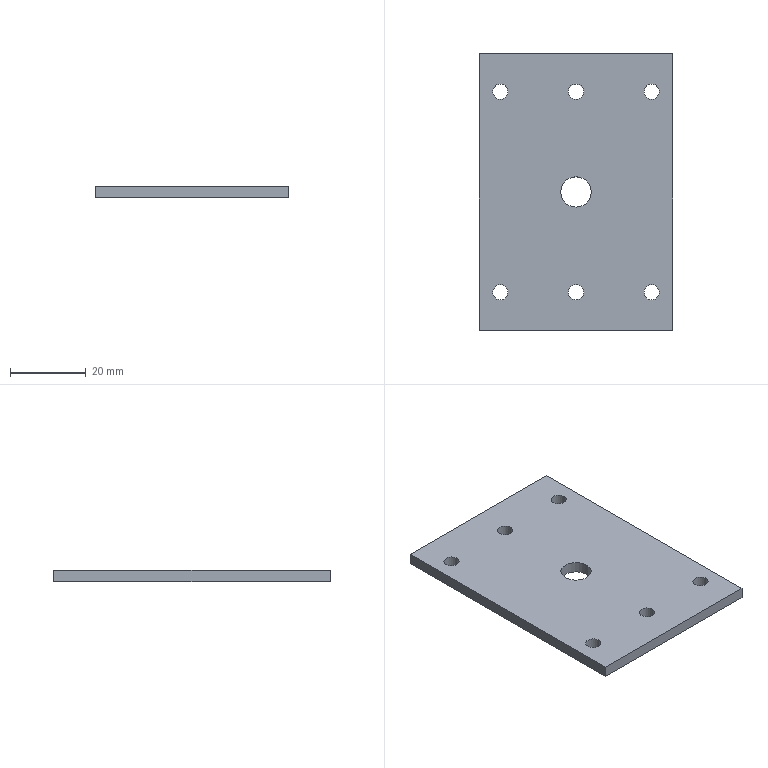Part | STEP file | 1-01.7 | 1 solid | 13 faces | box 51 x 73 x 3 mm | volume 10792 mm3 | cylinder 7 | plane 6 | commonest cylinder face diameters 4 x6 8 x1
STEP:
#1=CARTESIAN_POINT('',(0.,0.,0.));
#2=DIRECTION('',(0.,0.,1.));
#3=DIRECTION('',(1.,0.,0.));
#4=AXIS2_PLACEMENT_3D('',#1,#2,#3);
#5=CARTESIAN_POINT('',(25.5,-36.5,0.));
#6=VERTEX_POINT('',#5);
#7=CARTESIAN_POINT('',(25.5,36.5,0.));
#8=VERTEX_POINT('',#7);
#9=CARTESIAN_POINT('',(25.5,-36.5,0.));
#10=DIRECTION('',(0.,1.,0.));
#11=VECTOR('',#10,1.);
#12=LINE('',#9,#11);
#13=CARTESIAN_POINT('',(-11.,0.,0.));
#14=DIRECTION('',(0.,0.,1.));
#15=DIRECTION('',(0.,1.,0.));
#16=AXIS2_PLACEMENT_3D('',#13,#14,#15);
#17=PLANE('',#16);
#18=CARTESIAN_POINT('',(-36.5,-36.5));
#19=DIRECTION('',(1.,0.));
#20=VECTOR('',#19,1.);
#21=LINE('',#18,#20);
#22=(GEOMETRIC_REPRESENTATION_CONTEXT(2)PARAMETRIC_REPRESENTATION_CONTEXT()REPRESENTATION_CONTEXT('',''));
#23=DEFINITIONAL_REPRESENTATION('',(#21),#22);
#24=PCURVE('',#17,#23);
#25=CARTESIAN_POINT('',(25.5,0.,-1.5));
#26=DIRECTION('',(-1.,0.,0.));
#27=DIRECTION('',(0.,1.,0.));
#28=AXIS2_PLACEMENT_3D('',#25,#26,#27);
#29=PLANE('',#28);
#30=CARTESIAN_POINT('',(-36.5,-1.5));
#31=DIRECTION('',(1.,0.));
#32=VECTOR('',#31,1.);
#33=LINE('',#30,#32);
#34=(GEOMETRIC_REPRESENTATION_CONTEXT(2)PARAMETRIC_REPRESENTATION_CONTEXT()REPRESENTATION_CONTEXT('',''));
#35=DEFINITIONAL_REPRESENTATION('',(#33),#34);
#36=PCURVE('',#29,#35);
#37=SURFACE_CURVE('',#12,(#24,#36),.PCURVE_S1.);
#38=EDGE_CURVE('',#6,#8,#37,.T.);
#39=ORIENTED_EDGE('',*,*,#38,.T.);
#40=CARTESIAN_POINT('',(-25.5,36.5,0.));
#41=VERTEX_POINT('',#40);
#42=CARTESIAN_POINT('',(25.5,36.5,0.));
#43=DIRECTION('',(-1.,0.,0.));
#44=VECTOR('',#43,1.);
#45=LINE('',#42,#44);
#46=CARTESIAN_POINT('',(36.5,-36.5));
#47=DIRECTION('',(0.,1.));
#48=VECTOR('',#47,1.);
#49=LINE('',#46,#48);
#50=(GEOMETRIC_REPRESENTATION_CONTEXT(2)PARAMETRIC_REPRESENTATION_CONTEXT()REPRESENTATION_CONTEXT('',''));
#51=DEFINITIONAL_REPRESENTATION('',(#49),#50);
#52=PCURVE('',#17,#51);
#53=CARTESIAN_POINT('',(0.,36.5,-1.5));
#54=DIRECTION('',(0.,-1.,0.));
#55=DIRECTION('',(-1.,0.,0.));
#56=AXIS2_PLACEMENT_3D('',#53,#54,#55);
#57=PLANE('',#56);
#58=CARTESIAN_POINT('',(-25.5,-1.5));
#59=DIRECTION('',(1.,0.));
#60=VECTOR('',#59,1.);
#61=LINE('',#58,#60);
#62=(GEOMETRIC_REPRESENTATION_CONTEXT(2)PARAMETRIC_REPRESENTATION_CONTEXT()REPRESENTATION_CONTEXT('',''));
#63=DEFINITIONAL_REPRESENTATION('',(#61),#62);
#64=PCURVE('',#57,#63);
#65=SURFACE_CURVE('',#45,(#52,#64),.PCURVE_S1.);
#66=EDGE_CURVE('',#8,#41,#65,.T.);
#67=ORIENTED_EDGE('',*,*,#66,.T.);
#68=CARTESIAN_POINT('',(-25.5,-36.5,0.));
#69=VERTEX_POINT('',#68);
#70=CARTESIAN_POINT('',(-25.5,36.5,0.));
#71=DIRECTION('',(0.,-1.,0.));
#72=VECTOR('',#71,1.);
#73=LINE('',#70,#72);
#74=CARTESIAN_POINT('',(36.5,14.5));
#75=DIRECTION('',(-1.,0.));
#76=VECTOR('',#75,1.);
#77=LINE('',#74,#76);
#78=(GEOMETRIC_REPRESENTATION_CONTEXT(2)PARAMETRIC_REPRESENTATION_CONTEXT()REPRESENTATION_CONTEXT('',''));
#79=DEFINITIONAL_REPRESENTATION('',(#77),#78);
#80=PCURVE('',#17,#79);
#81=CARTESIAN_POINT('',(-25.5,0.,-1.5));
#82=DIRECTION('',(1.,0.,0.));
#83=DIRECTION('',(0.,-1.,0.));
#84=AXIS2_PLACEMENT_3D('',#81,#82,#83);
#85=PLANE('',#84);
#86=CARTESIAN_POINT('',(-36.5,-1.5));
#87=DIRECTION('',(1.,0.));
#88=VECTOR('',#87,1.);
#89=LINE('',#86,#88);
#90=(GEOMETRIC_REPRESENTATION_CONTEXT(2)PARAMETRIC_REPRESENTATION_CONTEXT()REPRESENTATION_CONTEXT('',''));
#91=DEFINITIONAL_REPRESENTATION('',(#89),#90);
#92=PCURVE('',#85,#91);
#93=SURFACE_CURVE('',#73,(#80,#92),.PCURVE_S1.);
#94=EDGE_CURVE('',#41,#69,#93,.T.);
#95=ORIENTED_EDGE('',*,*,#94,.T.);
#96=CARTESIAN_POINT('',(-25.5,-36.5,0.));
#97=DIRECTION('',(1.,0.,0.));
#98=VECTOR('',#97,1.);
#99=LINE('',#96,#98);
#100=CARTESIAN_POINT('',(-36.5,14.5));
#101=DIRECTION('',(0.,-1.));
#102=VECTOR('',#101,1.);
#103=LINE('',#100,#102);
#104=(GEOMETRIC_REPRESENTATION_CONTEXT(2)PARAMETRIC_REPRESENTATION_CONTEXT()REPRESENTATION_CONTEXT('',''));
#105=DEFINITIONAL_REPRESENTATION('',(#103),#104);
#106=PCURVE('',#17,#105);
#107=CARTESIAN_POINT('',(0.,-36.5,-1.5));
#108=DIRECTION('',(0.,1.,0.));
#109=DIRECTION('',(1.,0.,0.));
#110=AXIS2_PLACEMENT_3D('',#107,#108,#109);
#111=PLANE('',#110);
#112=CARTESIAN_POINT('',(-25.5,-1.5));
#113=DIRECTION('',(1.,0.));
#114=VECTOR('',#113,1.);
#115=LINE('',#112,#114);
#116=(GEOMETRIC_REPRESENTATION_CONTEXT(2)PARAMETRIC_REPRESENTATION_CONTEXT()REPRESENTATION_CONTEXT('',''));
#117=DEFINITIONAL_REPRESENTATION('',(#115),#116);
#118=PCURVE('',#111,#117);
#119=SURFACE_CURVE('',#99,(#106,#118),.PCURVE_S1.);
#120=EDGE_CURVE('',#69,#6,#119,.T.);
#121=ORIENTED_EDGE('',*,*,#120,.T.);
#122=EDGE_LOOP('',(#39,#67,#95,#121));
#123=FACE_BOUND('',#122,.T.);
#124=CARTESIAN_POINT('',(-20.,-24.5,0.));
#125=VERTEX_POINT('',#124);
#126=CARTESIAN_POINT('',(-20.,-26.5,0.));
#127=DIRECTION('',(0.,0.,-1.));
#128=DIRECTION('',(0.,1.,0.));
#129=AXIS2_PLACEMENT_3D('',#126,#127,#128);
#130=CIRCLE('',#129,2.);
#131=CARTESIAN_POINT('',(-24.5,9.));
#132=CARTESIAN_POINT('',(-24.5,5.536));
#133=CARTESIAN_POINT('',(-27.5,7.268));
#134=CARTESIAN_POINT('',(-30.5,9.));
#135=CARTESIAN_POINT('',(-27.5,10.732));
#136=CARTESIAN_POINT('',(-24.5,12.464));
#137=CARTESIAN_POINT('',(-24.5,9.));
#138=(BOUNDED_CURVE()B_SPLINE_CURVE(2,(#131,#132,#133,#134,#135,#136,#137),.UNSPECIFIED.,.T.,.F.)B_SPLINE_CURVE_WITH_KNOTS((1,2,2,2,2,1),(-2.094,0.,2.094,4.189,6.283,8.378),.UNSPECIFIED.)CURVE()GEOMETRIC_REPRESENTATION_ITEM()RATIONAL_B_SPLINE_CURVE((1.,0.5,1.,0.5,1.,0.5,1.))REPRESENTATION_ITEM(''));
#139=(GEOMETRIC_REPRESENTATION_CONTEXT(2)PARAMETRIC_REPRESENTATION_CONTEXT()REPRESENTATION_CONTEXT('',''));
#140=DEFINITIONAL_REPRESENTATION('',(#138),#139);
#141=PCURVE('',#17,#140);
#142=CARTESIAN_POINT('',(-20.,-26.5,0.));
#143=DIRECTION('',(0.,0.,-1.));
#144=DIRECTION('',(0.,1.,0.));
#145=AXIS2_PLACEMENT_3D('',#142,#143,#144);
#146=CYLINDRICAL_SURFACE('',#145,2.);
#147=CARTESIAN_POINT('',(0.,0.));
#148=DIRECTION('',(1.,0.));
#149=VECTOR('',#148,1.);
#150=LINE('',#147,#149);
#151=(GEOMETRIC_REPRESENTATION_CONTEXT(2)PARAMETRIC_REPRESENTATION_CONTEXT()REPRESENTATION_CONTEXT('',''));
#152=DEFINITIONAL_REPRESENTATION('',(#150),#151);
#153=PCURVE('',#146,#152);
#154=SURFACE_CURVE('',#130,(#141,#153),.PCURVE_S1.);
#155=EDGE_CURVE('',#125,#125,#154,.T.);
#156=ORIENTED_EDGE('',*,*,#155,.T.);
#157=EDGE_LOOP('',(#156));
#158=FACE_BOUND('',#157,.T.);
#159=CARTESIAN_POINT('',(0.,-24.5,0.));
#160=VERTEX_POINT('',#159);
#161=CARTESIAN_POINT('',(0.,-26.5,0.));
#162=DIRECTION('',(0.,0.,-1.));
#163=DIRECTION('',(0.,1.,0.));
#164=AXIS2_PLACEMENT_3D('',#161,#162,#163);
#165=CIRCLE('',#164,2.);
#166=CARTESIAN_POINT('',(-24.5,-11.));
#167=CARTESIAN_POINT('',(-24.5,-14.464));
#168=CARTESIAN_POINT('',(-27.5,-12.732));
#169=CARTESIAN_POINT('',(-30.5,-11.));
#170=CARTESIAN_POINT('',(-27.5,-9.268));
#171=CARTESIAN_POINT('',(-24.5,-7.536));
#172=CARTESIAN_POINT('',(-24.5,-11.));
#173=(BOUNDED_CURVE()B_SPLINE_CURVE(2,(#166,#167,#168,#169,#170,#171,#172),.UNSPECIFIED.,.T.,.F.)B_SPLINE_CURVE_WITH_KNOTS((1,2,2,2,2,1),(-2.094,0.,2.094,4.189,6.283,8.378),.UNSPECIFIED.)CURVE()GEOMETRIC_REPRESENTATION_ITEM()RATIONAL_B_SPLINE_CURVE((1.,0.5,1.,0.5,1.,0.5,1.))REPRESENTATION_ITEM(''));
#174=(GEOMETRIC_REPRESENTATION_CONTEXT(2)PARAMETRIC_REPRESENTATION_CONTEXT()REPRESENTATION_CONTEXT('',''));
#175=DEFINITIONAL_REPRESENTATION('',(#173),#174);
#176=PCURVE('',#17,#175);
#177=CARTESIAN_POINT('',(0.,-26.5,0.));
#178=DIRECTION('',(0.,0.,-1.));
#179=DIRECTION('',(0.,1.,0.));
#180=AXIS2_PLACEMENT_3D('',#177,#178,#179);
#181=CYLINDRICAL_SURFACE('',#180,2.);
#182=CARTESIAN_POINT('',(0.,0.));
#183=DIRECTION('',(1.,0.));
#184=VECTOR('',#183,1.);
#185=LINE('',#182,#184);
#186=(GEOMETRIC_REPRESENTATION_CONTEXT(2)PARAMETRIC_REPRESENTATION_CONTEXT()REPRESENTATION_CONTEXT('',''));
#187=DEFINITIONAL_REPRESENTATION('',(#185),#186);
#188=PCURVE('',#181,#187);
#189=SURFACE_CURVE('',#165,(#176,#188),.PCURVE_S1.);
#190=EDGE_CURVE('',#160,#160,#189,.T.);
#191=ORIENTED_EDGE('',*,*,#190,.T.);
#192=EDGE_LOOP('',(#191));
#193=FACE_BOUND('',#192,.T.);
#194=CARTESIAN_POINT('',(0.,4.,0.));
#195=VERTEX_POINT('',#194);
#196=CARTESIAN_POINT('',(0.,0.,0.));
#197=DIRECTION('',(0.,0.,-1.));
#198=DIRECTION('',(0.,1.,0.));
#199=AXIS2_PLACEMENT_3D('',#196,#197,#198);
#200=CIRCLE('',#199,4.);
#201=CARTESIAN_POINT('',(4.,-11.));
#202=CARTESIAN_POINT('',(4.,-17.928));
#203=CARTESIAN_POINT('',(-2.,-14.464));
#204=CARTESIAN_POINT('',(-8.,-11.));
#205=CARTESIAN_POINT('',(-2.,-7.536));
#206=CARTESIAN_POINT('',(4.,-4.072));
#207=CARTESIAN_POINT('',(4.,-11.));
#208=(BOUNDED_CURVE()B_SPLINE_CURVE(2,(#201,#202,#203,#204,#205,#206,#207),.UNSPECIFIED.,.T.,.F.)B_SPLINE_CURVE_WITH_KNOTS((1,2,2,2,2,1),(-2.094,0.,2.094,4.189,6.283,8.378),.UNSPECIFIED.)CURVE()GEOMETRIC_REPRESENTATION_ITEM()RATIONAL_B_SPLINE_CURVE((1.,0.5,1.,0.5,1.,0.5,1.))REPRESENTATION_ITEM(''));
#209=(GEOMETRIC_REPRESENTATION_CONTEXT(2)PARAMETRIC_REPRESENTATION_CONTEXT()REPRESENTATION_CONTEXT('',''));
#210=DEFINITIONAL_REPRESENTATION('',(#208),#209);
#211=PCURVE('',#17,#210);
#212=CARTESIAN_POINT('',(0.,0.,0.));
#213=DIRECTION('',(0.,0.,-1.));
#214=DIRECTION('',(0.,1.,0.));
#215=AXIS2_PLACEMENT_3D('',#212,#213,#214);
#216=CYLINDRICAL_SURFACE('',#215,4.);
#217=CARTESIAN_POINT('',(0.,0.));
#218=DIRECTION('',(1.,0.));
#219=VECTOR('',#218,1.);
#220=LINE('',#217,#219);
#221=(GEOMETRIC_REPRESENTATION_CONTEXT(2)PARAMETRIC_REPRESENTATION_CONTEXT()REPRESENTATION_CONTEXT('',''));
#222=DEFINITIONAL_REPRESENTATION('',(#220),#221);
#223=PCURVE('',#216,#222);
#224=SURFACE_CURVE('',#200,(#211,#223),.PCURVE_S1.);
#225=EDGE_CURVE('',#195,#195,#224,.T.);
#226=ORIENTED_EDGE('',*,*,#225,.T.);
#227=EDGE_LOOP('',(#226));
#228=FACE_BOUND('',#227,.T.);
#229=CARTESIAN_POINT('',(20.,-24.5,0.));
#230=VERTEX_POINT('',#229);
#231=CARTESIAN_POINT('',(20.,-26.5,0.));
#232=DIRECTION('',(0.,0.,-1.));
#233=DIRECTION('',(0.,1.,0.));
#234=AXIS2_PLACEMENT_3D('',#231,#232,#233);
#235=CIRCLE('',#234,2.);
#236=CARTESIAN_POINT('',(-24.5,-31.));
#237=CARTESIAN_POINT('',(-24.5,-34.464));
#238=CARTESIAN_POINT('',(-27.5,-32.732));
#239=CARTESIAN_POINT('',(-30.5,-31.));
#240=CARTESIAN_POINT('',(-27.5,-29.268));
#241=CARTESIAN_POINT('',(-24.5,-27.536));
#242=CARTESIAN_POINT('',(-24.5,-31.));
#243=(BOUNDED_CURVE()B_SPLINE_CURVE(2,(#236,#237,#238,#239,#240,#241,#242),.UNSPECIFIED.,.T.,.F.)B_SPLINE_CURVE_WITH_KNOTS((1,2,2,2,2,1),(-2.094,0.,2.094,4.189,6.283,8.378),.UNSPECIFIED.)CURVE()GEOMETRIC_REPRESENTATION_ITEM()RATIONAL_B_SPLINE_CURVE((1.,0.5,1.,0.5,1.,0.5,1.))REPRESENTATION_ITEM(''));
#244=(GEOMETRIC_REPRESENTATION_CONTEXT(2)PARAMETRIC_REPRESENTATION_CONTEXT()REPRESENTATION_CONTEXT('',''));
#245=DEFINITIONAL_REPRESENTATION('',(#243),#244);
#246=PCURVE('',#17,#245);
#247=CARTESIAN_POINT('',(20.,-26.5,0.));
#248=DIRECTION('',(0.,0.,-1.));
#249=DIRECTION('',(0.,1.,0.));
#250=AXIS2_PLACEMENT_3D('',#247,#248,#249);
#251=CYLINDRICAL_SURFACE('',#250,2.);
#252=CARTESIAN_POINT('',(0.,0.));
#253=DIRECTION('',(1.,0.));
#254=VECTOR('',#253,1.);
#255=LINE('',#252,#254);
#256=(GEOMETRIC_REPRESENTATION_CONTEXT(2)PARAMETRIC_REPRESENTATION_CONTEXT()REPRESENTATION_CONTEXT('',''));
#257=DEFINITIONAL_REPRESENTATION('',(#255),#256);
#258=PCURVE('',#251,#257);
#259=SURFACE_CURVE('',#235,(#246,#258),.PCURVE_S1.);
#260=EDGE_CURVE('',#230,#230,#259,.T.);
#261=ORIENTED_EDGE('',*,*,#260,.T.);
#262=EDGE_LOOP('',(#261));
#263=FACE_BOUND('',#262,.T.);
#264=CARTESIAN_POINT('',(-20.,28.5,0.));
#265=VERTEX_POINT('',#264);
#266=CARTESIAN_POINT('',(-20.,26.5,0.));
#267=DIRECTION('',(0.,0.,-1.));
#268=DIRECTION('',(0.,1.,0.));
#269=AXIS2_PLACEMENT_3D('',#266,#267,#268);
#270=CIRCLE('',#269,2.);
#271=CARTESIAN_POINT('',(28.5,9.));
#272=CARTESIAN_POINT('',(28.5,5.536));
#273=CARTESIAN_POINT('',(25.5,7.268));
#274=CARTESIAN_POINT('',(22.5,9.));
#275=CARTESIAN_POINT('',(25.5,10.732));
#276=CARTESIAN_POINT('',(28.5,12.464));
#277=CARTESIAN_POINT('',(28.5,9.));
#278=(BOUNDED_CURVE()B_SPLINE_CURVE(2,(#271,#272,#273,#274,#275,#276,#277),.UNSPECIFIED.,.T.,.F.)B_SPLINE_CURVE_WITH_KNOTS((1,2,2,2,2,1),(-2.094,0.,2.094,4.189,6.283,8.378),.UNSPECIFIED.)CURVE()GEOMETRIC_REPRESENTATION_ITEM()RATIONAL_B_SPLINE_CURVE((1.,0.5,1.,0.5,1.,0.5,1.))REPRESENTATION_ITEM(''));
#279=(GEOMETRIC_REPRESENTATION_CONTEXT(2)PARAMETRIC_REPRESENTATION_CONTEXT()REPRESENTATION_CONTEXT('',''));
#280=DEFINITIONAL_REPRESENTATION('',(#278),#279);
#281=PCURVE('',#17,#280);
#282=CARTESIAN_POINT('',(-20.,26.5,0.));
#283=DIRECTION('',(0.,0.,-1.));
#284=DIRECTION('',(0.,1.,0.));
#285=AXIS2_PLACEMENT_3D('',#282,#283,#284);
#286=CYLINDRICAL_SURFACE('',#285,2.);
#287=CARTESIAN_POINT('',(0.,0.));
#288=DIRECTION('',(1.,0.));
#289=VECTOR('',#288,1.);
#290=LINE('',#287,#289);
#291=(GEOMETRIC_REPRESENTATION_CONTEXT(2)PARAMETRIC_REPRESENTATION_CONTEXT()REPRESENTATION_CONTEXT('',''));
#292=DEFINITIONAL_REPRESENTATION('',(#290),#291);
#293=PCURVE('',#286,#292);
#294=SURFACE_CURVE('',#270,(#281,#293),.PCURVE_S1.);
#295=EDGE_CURVE('',#265,#265,#294,.T.);
#296=ORIENTED_EDGE('',*,*,#295,.T.);
#297=EDGE_LOOP('',(#296));
#298=FACE_BOUND('',#297,.T.);
#299=CARTESIAN_POINT('',(0.,28.5,0.));
#300=VERTEX_POINT('',#299);
#301=CARTESIAN_POINT('',(0.,26.5,0.));
#302=DIRECTION('',(0.,0.,-1.));
#303=DIRECTION('',(0.,1.,0.));
#304=AXIS2_PLACEMENT_3D('',#301,#302,#303);
#305=CIRCLE('',#304,2.);
#306=CARTESIAN_POINT('',(28.5,-11.));
#307=CARTESIAN_POINT('',(28.5,-14.464));
#308=CARTESIAN_POINT('',(25.5,-12.732));
#309=CARTESIAN_POINT('',(22.5,-11.));
#310=CARTESIAN_POINT('',(25.5,-9.268));
#311=CARTESIAN_POINT('',(28.5,-7.536));
#312=CARTESIAN_POINT('',(28.5,-11.));
#313=(BOUNDED_CURVE()B_SPLINE_CURVE(2,(#306,#307,#308,#309,#310,#311,#312),.UNSPECIFIED.,.T.,.F.)B_SPLINE_CURVE_WITH_KNOTS((1,2,2,2,2,1),(-2.094,0.,2.094,4.189,6.283,8.378),.UNSPECIFIED.)CURVE()GEOMETRIC_REPRESENTATION_ITEM()RATIONAL_B_SPLINE_CURVE((1.,0.5,1.,0.5,1.,0.5,1.))REPRESENTATION_ITEM(''));
#314=(GEOMETRIC_REPRESENTATION_CONTEXT(2)PARAMETRIC_REPRESENTATION_CONTEXT()REPRESENTATION_CONTEXT('',''));
#315=DEFINITIONAL_REPRESENTATION('',(#313),#314);
#316=PCURVE('',#17,#315);
#317=CARTESIAN_POINT('',(0.,26.5,0.));
#318=DIRECTION('',(0.,0.,-1.));
#319=DIRECTION('',(0.,1.,0.));
#320=AXIS2_PLACEMENT_3D('',#317,#318,#319);
#321=CYLINDRICAL_SURFACE('',#320,2.);
#322=CARTESIAN_POINT('',(0.,0.));
#323=DIRECTION('',(1.,0.));
#324=VECTOR('',#323,1.);
#325=LINE('',#322,#324);
#326=(GEOMETRIC_REPRESENTATION_CONTEXT(2)PARAMETRIC_REPRESENTATION_CONTEXT()REPRESENTATION_CONTEXT('',''));
#327=DEFINITIONAL_REPRESENTATION('',(#325),#326);
#328=PCURVE('',#321,#327);
#329=SURFACE_CURVE('',#305,(#316,#328),.PCURVE_S1.);
#330=EDGE_CURVE('',#300,#300,#329,.T.);
#331=ORIENTED_EDGE('',*,*,#330,.T.);
#332=EDGE_LOOP('',(#331));
#333=FACE_BOUND('',#332,.T.);
#334=CARTESIAN_POINT('',(20.,28.5,0.));
#335=VERTEX_POINT('',#334);
#336=CARTESIAN_POINT('',(20.,26.5,0.));
#337=DIRECTION('',(0.,0.,-1.));
#338=DIRECTION('',(0.,1.,0.));
#339=AXIS2_PLACEMENT_3D('',#336,#337,#338);
#340=CIRCLE('',#339,2.);
#341=CARTESIAN_POINT('',(28.5,-31.));
#342=CARTESIAN_POINT('',(28.5,-34.464));
#343=CARTESIAN_POINT('',(25.5,-32.732));
#344=CARTESIAN_POINT('',(22.5,-31.));
#345=CARTESIAN_POINT('',(25.5,-29.268));
#346=CARTESIAN_POINT('',(28.5,-27.536));
#347=CARTESIAN_POINT('',(28.5,-31.));
#348=(BOUNDED_CURVE()B_SPLINE_CURVE(2,(#341,#342,#343,#344,#345,#346,#347),.UNSPECIFIED.,.T.,.F.)B_SPLINE_CURVE_WITH_KNOTS((1,2,2,2,2,1),(-2.094,0.,2.094,4.189,6.283,8.378),.UNSPECIFIED.)CURVE()GEOMETRIC_REPRESENTATION_ITEM()RATIONAL_B_SPLINE_CURVE((1.,0.5,1.,0.5,1.,0.5,1.))REPRESENTATION_ITEM(''));
#349=(GEOMETRIC_REPRESENTATION_CONTEXT(2)PARAMETRIC_REPRESENTATION_CONTEXT()REPRESENTATION_CONTEXT('',''));
#350=DEFINITIONAL_REPRESENTATION('',(#348),#349);
#351=PCURVE('',#17,#350);
#352=CARTESIAN_POINT('',(20.,26.5,0.));
#353=DIRECTION('',(0.,0.,-1.));
#354=DIRECTION('',(0.,1.,0.));
#355=AXIS2_PLACEMENT_3D('',#352,#353,#354);
#356=CYLINDRICAL_SURFACE('',#355,2.);
#357=CARTESIAN_POINT('',(0.,0.));
#358=DIRECTION('',(1.,0.));
#359=VECTOR('',#358,1.);
#360=LINE('',#357,#359);
#361=(GEOMETRIC_REPRESENTATION_CONTEXT(2)PARAMETRIC_REPRESENTATION_CONTEXT()REPRESENTATION_CONTEXT('',''));
#362=DEFINITIONAL_REPRESENTATION('',(#360),#361);
#363=PCURVE('',#356,#362);
#364=SURFACE_CURVE('',#340,(#351,#363),.PCURVE_S1.);
#365=EDGE_CURVE('',#335,#335,#364,.T.);
#366=ORIENTED_EDGE('',*,*,#365,.T.);
#367=EDGE_LOOP('',(#366));
#368=FACE_BOUND('',#367,.T.);
#369=ADVANCED_FACE('',(#123,#158,#193,#228,#263,#298,#333,#368),#17,.T.);
#370=CARTESIAN_POINT('',(25.5,-36.5,-3.));
#371=VERTEX_POINT('',#370);
#372=CARTESIAN_POINT('',(25.5,36.5,-3.));
#373=VERTEX_POINT('',#372);
#374=CARTESIAN_POINT('',(25.5,-36.5,-3.));
#375=DIRECTION('',(0.,1.,0.));
#376=VECTOR('',#375,1.);
#377=LINE('',#374,#376);
#378=CARTESIAN_POINT('',(-11.,0.,-3.));
#379=DIRECTION('',(0.,0.,1.));
#380=DIRECTION('',(0.,1.,0.));
#381=AXIS2_PLACEMENT_3D('',#378,#379,#380);
#382=PLANE('',#381);
#383=CARTESIAN_POINT('',(-36.5,-36.5));
#384=DIRECTION('',(1.,0.));
#385=VECTOR('',#384,1.);
#386=LINE('',#383,#385);
#387=(GEOMETRIC_REPRESENTATION_CONTEXT(2)PARAMETRIC_REPRESENTATION_CONTEXT()REPRESENTATION_CONTEXT('',''));
#388=DEFINITIONAL_REPRESENTATION('',(#386),#387);
#389=PCURVE('',#382,#388);
#390=CARTESIAN_POINT('',(-36.5,1.5));
#391=DIRECTION('',(1.,0.));
#392=VECTOR('',#391,1.);
#393=LINE('',#390,#392);
#394=(GEOMETRIC_REPRESENTATION_CONTEXT(2)PARAMETRIC_REPRESENTATION_CONTEXT()REPRESENTATION_CONTEXT('',''));
#395=DEFINITIONAL_REPRESENTATION('',(#393),#394);
#396=PCURVE('',#29,#395);
#397=SURFACE_CURVE('',#377,(#389,#396),.PCURVE_S1.);
#398=EDGE_CURVE('',#371,#373,#397,.T.);
#399=ORIENTED_EDGE('',*,*,#398,.T.);
#400=CARTESIAN_POINT('',(-25.5,36.5,-3.));
#401=VERTEX_POINT('',#400);
#402=CARTESIAN_POINT('',(25.5,36.5,-3.));
#403=DIRECTION('',(-1.,0.,0.));
#404=VECTOR('',#403,1.);
#405=LINE('',#402,#404);
#406=CARTESIAN_POINT('',(36.5,-36.5));
#407=DIRECTION('',(0.,1.));
#408=VECTOR('',#407,1.);
#409=LINE('',#406,#408);
#410=(GEOMETRIC_REPRESENTATION_CONTEXT(2)PARAMETRIC_REPRESENTATION_CONTEXT()REPRESENTATION_CONTEXT('',''));
#411=DEFINITIONAL_REPRESENTATION('',(#409),#410);
#412=PCURVE('',#382,#411);
#413=CARTESIAN_POINT('',(-25.5,1.5));
#414=DIRECTION('',(1.,0.));
#415=VECTOR('',#414,1.);
#416=LINE('',#413,#415);
#417=(GEOMETRIC_REPRESENTATION_CONTEXT(2)PARAMETRIC_REPRESENTATION_CONTEXT()REPRESENTATION_CONTEXT('',''));
#418=DEFINITIONAL_REPRESENTATION('',(#416),#417);
#419=PCURVE('',#57,#418);
#420=SURFACE_CURVE('',#405,(#412,#419),.PCURVE_S1.);
#421=EDGE_CURVE('',#373,#401,#420,.T.);
#422=ORIENTED_EDGE('',*,*,#421,.T.);
#423=CARTESIAN_POINT('',(-25.5,-36.5,-3.));
#424=VERTEX_POINT('',#423);
#425=CARTESIAN_POINT('',(-25.5,36.5,-3.));
#426=DIRECTION('',(0.,-1.,0.));
#427=VECTOR('',#426,1.);
#428=LINE('',#425,#427);
#429=CARTESIAN_POINT('',(36.5,14.5));
#430=DIRECTION('',(-1.,0.));
#431=VECTOR('',#430,1.);
#432=LINE('',#429,#431);
#433=(GEOMETRIC_REPRESENTATION_CONTEXT(2)PARAMETRIC_REPRESENTATION_CONTEXT()REPRESENTATION_CONTEXT('',''));
#434=DEFINITIONAL_REPRESENTATION('',(#432),#433);
#435=PCURVE('',#382,#434);
#436=CARTESIAN_POINT('',(-36.5,1.5));
#437=DIRECTION('',(1.,0.));
#438=VECTOR('',#437,1.);
#439=LINE('',#436,#438);
#440=(GEOMETRIC_REPRESENTATION_CONTEXT(2)PARAMETRIC_REPRESENTATION_CONTEXT()REPRESENTATION_CONTEXT('',''));
#441=DEFINITIONAL_REPRESENTATION('',(#439),#440);
#442=PCURVE('',#85,#441);
#443=SURFACE_CURVE('',#428,(#435,#442),.PCURVE_S1.);
#444=EDGE_CURVE('',#401,#424,#443,.T.);
#445=ORIENTED_EDGE('',*,*,#444,.T.);
#446=CARTESIAN_POINT('',(-25.5,-36.5,-3.));
#447=DIRECTION('',(1.,0.,0.));
#448=VECTOR('',#447,1.);
#449=LINE('',#446,#448);
#450=CARTESIAN_POINT('',(-36.5,14.5));
#451=DIRECTION('',(0.,-1.));
#452=VECTOR('',#451,1.);
#453=LINE('',#450,#452);
#454=(GEOMETRIC_REPRESENTATION_CONTEXT(2)PARAMETRIC_REPRESENTATION_CONTEXT()REPRESENTATION_CONTEXT('',''));
#455=DEFINITIONAL_REPRESENTATION('',(#453),#454);
#456=PCURVE('',#382,#455);
#457=CARTESIAN_POINT('',(-25.5,1.5));
#458=DIRECTION('',(1.,0.));
#459=VECTOR('',#458,1.);
#460=LINE('',#457,#459);
#461=(GEOMETRIC_REPRESENTATION_CONTEXT(2)PARAMETRIC_REPRESENTATION_CONTEXT()REPRESENTATION_CONTEXT('',''));
#462=DEFINITIONAL_REPRESENTATION('',(#460),#461);
#463=PCURVE('',#111,#462);
#464=SURFACE_CURVE('',#449,(#456,#463),.PCURVE_S1.);
#465=EDGE_CURVE('',#424,#371,#464,.T.);
#466=ORIENTED_EDGE('',*,*,#465,.T.);
#467=EDGE_LOOP('',(#399,#422,#445,#466));
#468=FACE_BOUND('',#467,.F.);
#469=CARTESIAN_POINT('',(-20.,-24.5,-3.));
#470=VERTEX_POINT('',#469);
#471=CARTESIAN_POINT('',(-20.,-26.5,-3.));
#472=DIRECTION('',(0.,0.,-1.));
#473=DIRECTION('',(0.,1.,0.));
#474=AXIS2_PLACEMENT_3D('',#471,#472,#473);
#475=CIRCLE('',#474,2.);
#476=CARTESIAN_POINT('',(-24.5,9.));
#477=CARTESIAN_POINT('',(-24.5,5.536));
#478=CARTESIAN_POINT('',(-27.5,7.268));
#479=CARTESIAN_POINT('',(-30.5,9.));
#480=CARTESIAN_POINT('',(-27.5,10.732));
#481=CARTESIAN_POINT('',(-24.5,12.464));
#482=CARTESIAN_POINT('',(-24.5,9.));
#483=(BOUNDED_CURVE()B_SPLINE_CURVE(2,(#476,#477,#478,#479,#480,#481,#482),.UNSPECIFIED.,.T.,.F.)B_SPLINE_CURVE_WITH_KNOTS((1,2,2,2,2,1),(-2.094,0.,2.094,4.189,6.283,8.378),.UNSPECIFIED.)CURVE()GEOMETRIC_REPRESENTATION_ITEM()RATIONAL_B_SPLINE_CURVE((1.,0.5,1.,0.5,1.,0.5,1.))REPRESENTATION_ITEM(''));
#484=(GEOMETRIC_REPRESENTATION_CONTEXT(2)PARAMETRIC_REPRESENTATION_CONTEXT()REPRESENTATION_CONTEXT('',''));
#485=DEFINITIONAL_REPRESENTATION('',(#483),#484);
#486=PCURVE('',#382,#485);
#487=CARTESIAN_POINT('',(0.,3.));
#488=DIRECTION('',(1.,0.));
#489=VECTOR('',#488,1.);
#490=LINE('',#487,#489);
#491=(GEOMETRIC_REPRESENTATION_CONTEXT(2)PARAMETRIC_REPRESENTATION_CONTEXT()REPRESENTATION_CONTEXT('',''));
#492=DEFINITIONAL_REPRESENTATION('',(#490),#491);
#493=PCURVE('',#146,#492);
#494=SURFACE_CURVE('',#475,(#486,#493),.PCURVE_S1.);
#495=EDGE_CURVE('',#470,#470,#494,.T.);
#496=ORIENTED_EDGE('',*,*,#495,.T.);
#497=EDGE_LOOP('',(#496));
#498=FACE_BOUND('',#497,.F.);
#499=CARTESIAN_POINT('',(0.,-24.5,-3.));
#500=VERTEX_POINT('',#499);
#501=CARTESIAN_POINT('',(0.,-26.5,-3.));
#502=DIRECTION('',(0.,0.,-1.));
#503=DIRECTION('',(0.,1.,0.));
#504=AXIS2_PLACEMENT_3D('',#501,#502,#503);
#505=CIRCLE('',#504,2.);
#506=CARTESIAN_POINT('',(-24.5,-11.));
#507=CARTESIAN_POINT('',(-24.5,-14.464));
#508=CARTESIAN_POINT('',(-27.5,-12.732));
#509=CARTESIAN_POINT('',(-30.5,-11.));
#510=CARTESIAN_POINT('',(-27.5,-9.268));
#511=CARTESIAN_POINT('',(-24.5,-7.536));
#512=CARTESIAN_POINT('',(-24.5,-11.));
#513=(BOUNDED_CURVE()B_SPLINE_CURVE(2,(#506,#507,#508,#509,#510,#511,#512),.UNSPECIFIED.,.T.,.F.)B_SPLINE_CURVE_WITH_KNOTS((1,2,2,2,2,1),(-2.094,0.,2.094,4.189,6.283,8.378),.UNSPECIFIED.)CURVE()GEOMETRIC_REPRESENTATION_ITEM()RATIONAL_B_SPLINE_CURVE((1.,0.5,1.,0.5,1.,0.5,1.))REPRESENTATION_ITEM(''));
#514=(GEOMETRIC_REPRESENTATION_CONTEXT(2)PARAMETRIC_REPRESENTATION_CONTEXT()REPRESENTATION_CONTEXT('',''));
#515=DEFINITIONAL_REPRESENTATION('',(#513),#514);
#516=PCURVE('',#382,#515);
#517=CARTESIAN_POINT('',(0.,3.));
#518=DIRECTION('',(1.,0.));
#519=VECTOR('',#518,1.);
#520=LINE('',#517,#519);
#521=(GEOMETRIC_REPRESENTATION_CONTEXT(2)PARAMETRIC_REPRESENTATION_CONTEXT()REPRESENTATION_CONTEXT('',''));
#522=DEFINITIONAL_REPRESENTATION('',(#520),#521);
#523=PCURVE('',#181,#522);
#524=SURFACE_CURVE('',#505,(#516,#523),.PCURVE_S1.);
#525=EDGE_CURVE('',#500,#500,#524,.T.);
#526=ORIENTED_EDGE('',*,*,#525,.T.);
#527=EDGE_LOOP('',(#526));
#528=FACE_BOUND('',#527,.F.);
#529=CARTESIAN_POINT('',(0.,4.,-3.));
#530=VERTEX_POINT('',#529);
#531=CARTESIAN_POINT('',(0.,0.,-3.));
#532=DIRECTION('',(0.,0.,-1.));
#533=DIRECTION('',(0.,1.,0.));
#534=AXIS2_PLACEMENT_3D('',#531,#532,#533);
#535=CIRCLE('',#534,4.);
#536=CARTESIAN_POINT('',(4.,-11.));
#537=CARTESIAN_POINT('',(4.,-17.928));
#538=CARTESIAN_POINT('',(-2.,-14.464));
#539=CARTESIAN_POINT('',(-8.,-11.));
#540=CARTESIAN_POINT('',(-2.,-7.536));
#541=CARTESIAN_POINT('',(4.,-4.072));
#542=CARTESIAN_POINT('',(4.,-11.));
#543=(BOUNDED_CURVE()B_SPLINE_CURVE(2,(#536,#537,#538,#539,#540,#541,#542),.UNSPECIFIED.,.T.,.F.)B_SPLINE_CURVE_WITH_KNOTS((1,2,2,2,2,1),(-2.094,0.,2.094,4.189,6.283,8.378),.UNSPECIFIED.)CURVE()GEOMETRIC_REPRESENTATION_ITEM()RATIONAL_B_SPLINE_CURVE((1.,0.5,1.,0.5,1.,0.5,1.))REPRESENTATION_ITEM(''));
#544=(GEOMETRIC_REPRESENTATION_CONTEXT(2)PARAMETRIC_REPRESENTATION_CONTEXT()REPRESENTATION_CONTEXT('',''));
#545=DEFINITIONAL_REPRESENTATION('',(#543),#544);
#546=PCURVE('',#382,#545);
#547=CARTESIAN_POINT('',(0.,3.));
#548=DIRECTION('',(1.,0.));
#549=VECTOR('',#548,1.);
#550=LINE('',#547,#549);
#551=(GEOMETRIC_REPRESENTATION_CONTEXT(2)PARAMETRIC_REPRESENTATION_CONTEXT()REPRESENTATION_CONTEXT('',''));
#552=DEFINITIONAL_REPRESENTATION('',(#550),#551);
#553=PCURVE('',#216,#552);
#554=SURFACE_CURVE('',#535,(#546,#553),.PCURVE_S1.);
#555=EDGE_CURVE('',#530,#530,#554,.T.);
#556=ORIENTED_EDGE('',*,*,#555,.T.);
#557=EDGE_LOOP('',(#556));
#558=FACE_BOUND('',#557,.F.);
#559=CARTESIAN_POINT('',(20.,-24.5,-3.));
#560=VERTEX_POINT('',#559);
#561=CARTESIAN_POINT('',(20.,-26.5,-3.));
#562=DIRECTION('',(0.,0.,-1.));
#563=DIRECTION('',(0.,1.,0.));
#564=AXIS2_PLACEMENT_3D('',#561,#562,#563);
#565=CIRCLE('',#564,2.);
#566=CARTESIAN_POINT('',(-24.5,-31.));
#567=CARTESIAN_POINT('',(-24.5,-34.464));
#568=CARTESIAN_POINT('',(-27.5,-32.732));
#569=CARTESIAN_POINT('',(-30.5,-31.));
#570=CARTESIAN_POINT('',(-27.5,-29.268));
#571=CARTESIAN_POINT('',(-24.5,-27.536));
#572=CARTESIAN_POINT('',(-24.5,-31.));
#573=(BOUNDED_CURVE()B_SPLINE_CURVE(2,(#566,#567,#568,#569,#570,#571,#572),.UNSPECIFIED.,.T.,.F.)B_SPLINE_CURVE_WITH_KNOTS((1,2,2,2,2,1),(-2.094,0.,2.094,4.189,6.283,8.378),.UNSPECIFIED.)CURVE()GEOMETRIC_REPRESENTATION_ITEM()RATIONAL_B_SPLINE_CURVE((1.,0.5,1.,0.5,1.,0.5,1.))REPRESENTATION_ITEM(''));
#574=(GEOMETRIC_REPRESENTATION_CONTEXT(2)PARAMETRIC_REPRESENTATION_CONTEXT()REPRESENTATION_CONTEXT('',''));
#575=DEFINITIONAL_REPRESENTATION('',(#573),#574);
#576=PCURVE('',#382,#575);
#577=CARTESIAN_POINT('',(0.,3.));
#578=DIRECTION('',(1.,0.));
#579=VECTOR('',#578,1.);
#580=LINE('',#577,#579);
#581=(GEOMETRIC_REPRESENTATION_CONTEXT(2)PARAMETRIC_REPRESENTATION_CONTEXT()REPRESENTATION_CONTEXT('',''));
#582=DEFINITIONAL_REPRESENTATION('',(#580),#581);
#583=PCURVE('',#251,#582);
#584=SURFACE_CURVE('',#565,(#576,#583),.PCURVE_S1.);
#585=EDGE_CURVE('',#560,#560,#584,.T.);
#586=ORIENTED_EDGE('',*,*,#585,.T.);
#587=EDGE_LOOP('',(#586));
#588=FACE_BOUND('',#587,.F.);
#589=CARTESIAN_POINT('',(-20.,28.5,-3.));
#590=VERTEX_POINT('',#589);
#591=CARTESIAN_POINT('',(-20.,26.5,-3.));
#592=DIRECTION('',(0.,0.,-1.));
#593=DIRECTION('',(0.,1.,0.));
#594=AXIS2_PLACEMENT_3D('',#591,#592,#593);
#595=CIRCLE('',#594,2.);
#596=CARTESIAN_POINT('',(28.5,9.));
#597=CARTESIAN_POINT('',(28.5,5.536));
#598=CARTESIAN_POINT('',(25.5,7.268));
#599=CARTESIAN_POINT('',(22.5,9.));
#600=CARTESIAN_POINT('',(25.5,10.732));
#601=CARTESIAN_POINT('',(28.5,12.464));
#602=CARTESIAN_POINT('',(28.5,9.));
#603=(BOUNDED_CURVE()B_SPLINE_CURVE(2,(#596,#597,#598,#599,#600,#601,#602),.UNSPECIFIED.,.T.,.F.)B_SPLINE_CURVE_WITH_KNOTS((1,2,2,2,2,1),(-2.094,0.,2.094,4.189,6.283,8.378),.UNSPECIFIED.)CURVE()GEOMETRIC_REPRESENTATION_ITEM()RATIONAL_B_SPLINE_CURVE((1.,0.5,1.,0.5,1.,0.5,1.))REPRESENTATION_ITEM(''));
#604=(GEOMETRIC_REPRESENTATION_CONTEXT(2)PARAMETRIC_REPRESENTATION_CONTEXT()REPRESENTATION_CONTEXT('',''));
#605=DEFINITIONAL_REPRESENTATION('',(#603),#604);
#606=PCURVE('',#382,#605);
#607=CARTESIAN_POINT('',(0.,3.));
#608=DIRECTION('',(1.,0.));
#609=VECTOR('',#608,1.);
#610=LINE('',#607,#609);
#611=(GEOMETRIC_REPRESENTATION_CONTEXT(2)PARAMETRIC_REPRESENTATION_CONTEXT()REPRESENTATION_CONTEXT('',''));
#612=DEFINITIONAL_REPRESENTATION('',(#610),#611);
#613=PCURVE('',#286,#612);
#614=SURFACE_CURVE('',#595,(#606,#613),.PCURVE_S1.);
#615=EDGE_CURVE('',#590,#590,#614,.T.);
#616=ORIENTED_EDGE('',*,*,#615,.T.);
#617=EDGE_LOOP('',(#616));
#618=FACE_BOUND('',#617,.F.);
#619=CARTESIAN_POINT('',(0.,28.5,-3.));
#620=VERTEX_POINT('',#619);
#621=CARTESIAN_POINT('',(0.,26.5,-3.));
#622=DIRECTION('',(0.,0.,-1.));
#623=DIRECTION('',(0.,1.,0.));
#624=AXIS2_PLACEMENT_3D('',#621,#622,#623);
#625=CIRCLE('',#624,2.);
#626=CARTESIAN_POINT('',(28.5,-11.));
#627=CARTESIAN_POINT('',(28.5,-14.464));
#628=CARTESIAN_POINT('',(25.5,-12.732));
#629=CARTESIAN_POINT('',(22.5,-11.));
#630=CARTESIAN_POINT('',(25.5,-9.268));
#631=CARTESIAN_POINT('',(28.5,-7.536));
#632=CARTESIAN_POINT('',(28.5,-11.));
#633=(BOUNDED_CURVE()B_SPLINE_CURVE(2,(#626,#627,#628,#629,#630,#631,#632),.UNSPECIFIED.,.T.,.F.)B_SPLINE_CURVE_WITH_KNOTS((1,2,2,2,2,1),(-2.094,0.,2.094,4.189,6.283,8.378),.UNSPECIFIED.)CURVE()GEOMETRIC_REPRESENTATION_ITEM()RATIONAL_B_SPLINE_CURVE((1.,0.5,1.,0.5,1.,0.5,1.))REPRESENTATION_ITEM(''));
#634=(GEOMETRIC_REPRESENTATION_CONTEXT(2)PARAMETRIC_REPRESENTATION_CONTEXT()REPRESENTATION_CONTEXT('',''));
#635=DEFINITIONAL_REPRESENTATION('',(#633),#634);
#636=PCURVE('',#382,#635);
#637=CARTESIAN_POINT('',(0.,3.));
#638=DIRECTION('',(1.,0.));
#639=VECTOR('',#638,1.);
#640=LINE('',#637,#639);
#641=(GEOMETRIC_REPRESENTATION_CONTEXT(2)PARAMETRIC_REPRESENTATION_CONTEXT()REPRESENTATION_CONTEXT('',''));
#642=DEFINITIONAL_REPRESENTATION('',(#640),#641);
#643=PCURVE('',#321,#642);
#644=SURFACE_CURVE('',#625,(#636,#643),.PCURVE_S1.);
#645=EDGE_CURVE('',#620,#620,#644,.T.);
#646=ORIENTED_EDGE('',*,*,#645,.T.);
#647=EDGE_LOOP('',(#646));
#648=FACE_BOUND('',#647,.F.);
#649=CARTESIAN_POINT('',(20.,28.5,-3.));
#650=VERTEX_POINT('',#649);
#651=CARTESIAN_POINT('',(20.,26.5,-3.));
#652=DIRECTION('',(0.,0.,-1.));
#653=DIRECTION('',(0.,1.,0.));
#654=AXIS2_PLACEMENT_3D('',#651,#652,#653);
#655=CIRCLE('',#654,2.);
#656=CARTESIAN_POINT('',(28.5,-31.));
#657=CARTESIAN_POINT('',(28.5,-34.464));
#658=CARTESIAN_POINT('',(25.5,-32.732));
#659=CARTESIAN_POINT('',(22.5,-31.));
#660=CARTESIAN_POINT('',(25.5,-29.268));
#661=CARTESIAN_POINT('',(28.5,-27.536));
#662=CARTESIAN_POINT('',(28.5,-31.));
#663=(BOUNDED_CURVE()B_SPLINE_CURVE(2,(#656,#657,#658,#659,#660,#661,#662),.UNSPECIFIED.,.T.,.F.)B_SPLINE_CURVE_WITH_KNOTS((1,2,2,2,2,1),(-2.094,0.,2.094,4.189,6.283,8.378),.UNSPECIFIED.)CURVE()GEOMETRIC_REPRESENTATION_ITEM()RATIONAL_B_SPLINE_CURVE((1.,0.5,1.,0.5,1.,0.5,1.))REPRESENTATION_ITEM(''));
#664=(GEOMETRIC_REPRESENTATION_CONTEXT(2)PARAMETRIC_REPRESENTATION_CONTEXT()REPRESENTATION_CONTEXT('',''));
#665=DEFINITIONAL_REPRESENTATION('',(#663),#664);
#666=PCURVE('',#382,#665);
#667=CARTESIAN_POINT('',(0.,3.));
#668=DIRECTION('',(1.,0.));
#669=VECTOR('',#668,1.);
#670=LINE('',#667,#669);
#671=(GEOMETRIC_REPRESENTATION_CONTEXT(2)PARAMETRIC_REPRESENTATION_CONTEXT()REPRESENTATION_CONTEXT('',''));
#672=DEFINITIONAL_REPRESENTATION('',(#670),#671);
#673=PCURVE('',#356,#672);
#674=SURFACE_CURVE('',#655,(#666,#673),.PCURVE_S1.);
#675=EDGE_CURVE('',#650,#650,#674,.T.);
#676=ORIENTED_EDGE('',*,*,#675,.T.);
#677=EDGE_LOOP('',(#676));
#678=FACE_BOUND('',#677,.F.);
#679=ADVANCED_FACE('',(#468,#498,#528,#558,#588,#618,#648,#678),#382,.F.);
#680=ORIENTED_EDGE('',*,*,#38,.T.);
#681=CARTESIAN_POINT('',(25.5,36.5,0.));
#682=DIRECTION('',(0.,0.,-1.));
#683=VECTOR('',#682,1.);
#684=LINE('',#681,#683);
#685=CARTESIAN_POINT('',(36.5,-1.5));
#686=DIRECTION('',(0.,1.));
#687=VECTOR('',#686,1.);
#688=LINE('',#685,#687);
#689=(GEOMETRIC_REPRESENTATION_CONTEXT(2)PARAMETRIC_REPRESENTATION_CONTEXT()REPRESENTATION_CONTEXT('',''));
#690=DEFINITIONAL_REPRESENTATION('',(#688),#689);
#691=PCURVE('',#29,#690);
#692=CARTESIAN_POINT('',(-25.5,-1.5));
#693=DIRECTION('',(0.,1.));
#694=VECTOR('',#693,1.);
#695=LINE('',#692,#694);
#696=(GEOMETRIC_REPRESENTATION_CONTEXT(2)PARAMETRIC_REPRESENTATION_CONTEXT()REPRESENTATION_CONTEXT('',''));
#697=DEFINITIONAL_REPRESENTATION('',(#695),#696);
#698=PCURVE('',#57,#697);
#699=SURFACE_CURVE('',#684,(#691,#698),.PCURVE_S1.);
#700=EDGE_CURVE('',#8,#373,#699,.T.);
#701=ORIENTED_EDGE('',*,*,#700,.T.);
#702=ORIENTED_EDGE('',*,*,#398,.F.);
#703=CARTESIAN_POINT('',(25.5,-36.5,0.));
#704=DIRECTION('',(0.,0.,-1.));
#705=VECTOR('',#704,1.);
#706=LINE('',#703,#705);
#707=CARTESIAN_POINT('',(-36.5,-1.5));
#708=DIRECTION('',(0.,1.));
#709=VECTOR('',#708,1.);
#710=LINE('',#707,#709);
#711=(GEOMETRIC_REPRESENTATION_CONTEXT(2)PARAMETRIC_REPRESENTATION_CONTEXT()REPRESENTATION_CONTEXT('',''));
#712=DEFINITIONAL_REPRESENTATION('',(#710),#711);
#713=PCURVE('',#29,#712);
#714=CARTESIAN_POINT('',(25.5,-1.5));
#715=DIRECTION('',(0.,1.));
#716=VECTOR('',#715,1.);
#717=LINE('',#714,#716);
#718=(GEOMETRIC_REPRESENTATION_CONTEXT(2)PARAMETRIC_REPRESENTATION_CONTEXT()REPRESENTATION_CONTEXT('',''));
#719=DEFINITIONAL_REPRESENTATION('',(#717),#718);
#720=PCURVE('',#111,#719);
#721=SURFACE_CURVE('',#706,(#713,#720),.PCURVE_S1.);
#722=EDGE_CURVE('',#6,#371,#721,.T.);
#723=ORIENTED_EDGE('',*,*,#722,.F.);
#724=EDGE_LOOP('',(#680,#701,#702,#723));
#725=FACE_BOUND('',#724,.F.);
#726=ADVANCED_FACE('',(#725),#29,.F.);
#727=ORIENTED_EDGE('',*,*,#66,.T.);
#728=CARTESIAN_POINT('',(-25.5,36.5,0.));
#729=DIRECTION('',(0.,0.,-1.));
#730=VECTOR('',#729,1.);
#731=LINE('',#728,#730);
#732=CARTESIAN_POINT('',(25.5,-1.5));
#733=DIRECTION('',(0.,1.));
#734=VECTOR('',#733,1.);
#735=LINE('',#732,#734);
#736=(GEOMETRIC_REPRESENTATION_CONTEXT(2)PARAMETRIC_REPRESENTATION_CONTEXT()REPRESENTATION_CONTEXT('',''));
#737=DEFINITIONAL_REPRESENTATION('',(#735),#736);
#738=PCURVE('',#57,#737);
#739=CARTESIAN_POINT('',(-36.5,-1.5));
#740=DIRECTION('',(0.,1.));
#741=VECTOR('',#740,1.);
#742=LINE('',#739,#741);
#743=(GEOMETRIC_REPRESENTATION_CONTEXT(2)PARAMETRIC_REPRESENTATION_CONTEXT()REPRESENTATION_CONTEXT('',''));
#744=DEFINITIONAL_REPRESENTATION('',(#742),#743);
#745=PCURVE('',#85,#744);
#746=SURFACE_CURVE('',#731,(#738,#745),.PCURVE_S1.);
#747=EDGE_CURVE('',#41,#401,#746,.T.);
#748=ORIENTED_EDGE('',*,*,#747,.T.);
#749=ORIENTED_EDGE('',*,*,#421,.F.);
#750=ORIENTED_EDGE('',*,*,#700,.F.);
#751=EDGE_LOOP('',(#727,#748,#749,#750));
#752=FACE_BOUND('',#751,.F.);
#753=ADVANCED_FACE('',(#752),#57,.F.);
#754=ORIENTED_EDGE('',*,*,#94,.T.);
#755=CARTESIAN_POINT('',(-25.5,-36.5,0.));
#756=DIRECTION('',(0.,0.,-1.));
#757=VECTOR('',#756,1.);
#758=LINE('',#755,#757);
#759=CARTESIAN_POINT('',(36.5,-1.5));
#760=DIRECTION('',(0.,1.));
#761=VECTOR('',#760,1.);
#762=LINE('',#759,#761);
#763=(GEOMETRIC_REPRESENTATION_CONTEXT(2)PARAMETRIC_REPRESENTATION_CONTEXT()REPRESENTATION_CONTEXT('',''));
#764=DEFINITIONAL_REPRESENTATION('',(#762),#763);
#765=PCURVE('',#85,#764);
#766=CARTESIAN_POINT('',(-25.5,-1.5));
#767=DIRECTION('',(0.,1.));
#768=VECTOR('',#767,1.);
#769=LINE('',#766,#768);
#770=(GEOMETRIC_REPRESENTATION_CONTEXT(2)PARAMETRIC_REPRESENTATION_CONTEXT()REPRESENTATION_CONTEXT('',''));
#771=DEFINITIONAL_REPRESENTATION('',(#769),#770);
#772=PCURVE('',#111,#771);
#773=SURFACE_CURVE('',#758,(#765,#772),.PCURVE_S1.);
#774=EDGE_CURVE('',#69,#424,#773,.T.);
#775=ORIENTED_EDGE('',*,*,#774,.T.);
#776=ORIENTED_EDGE('',*,*,#444,.F.);
#777=ORIENTED_EDGE('',*,*,#747,.F.);
#778=EDGE_LOOP('',(#754,#775,#776,#777));
#779=FACE_BOUND('',#778,.F.);
#780=ADVANCED_FACE('',(#779),#85,.F.);
#781=ORIENTED_EDGE('',*,*,#120,.T.);
#782=ORIENTED_EDGE('',*,*,#722,.T.);
#783=ORIENTED_EDGE('',*,*,#465,.F.);
#784=ORIENTED_EDGE('',*,*,#774,.F.);
#785=EDGE_LOOP('',(#781,#782,#783,#784));
#786=FACE_BOUND('',#785,.F.);
#787=ADVANCED_FACE('',(#786),#111,.F.);
#788=ORIENTED_EDGE('',*,*,#155,.T.);
#789=CARTESIAN_POINT('',(-20.,-24.5,0.));
#790=DIRECTION('',(0.,0.,-1.));
#791=VECTOR('',#790,1.);
#792=LINE('',#789,#791);
#793=CARTESIAN_POINT('',(6.283,0.));
#794=DIRECTION('',(0.,1.));
#795=VECTOR('',#794,1.);
#796=LINE('',#793,#795);
#797=(GEOMETRIC_REPRESENTATION_CONTEXT(2)PARAMETRIC_REPRESENTATION_CONTEXT()REPRESENTATION_CONTEXT('',''));
#798=DEFINITIONAL_REPRESENTATION('',(#796),#797);
#799=PCURVE('',#146,#798);
#800=CARTESIAN_POINT('',(0.,0.));
#801=DIRECTION('',(0.,1.));
#802=VECTOR('',#801,1.);
#803=LINE('',#800,#802);
#804=(GEOMETRIC_REPRESENTATION_CONTEXT(2)PARAMETRIC_REPRESENTATION_CONTEXT()REPRESENTATION_CONTEXT('',''));
#805=DEFINITIONAL_REPRESENTATION('',(#803),#804);
#806=PCURVE('',#146,#805);
#807=SEAM_CURVE('',#792,(#799,#806),.PCURVE_S1.);
#808=EDGE_CURVE('',#125,#470,#807,.T.);
#809=ORIENTED_EDGE('',*,*,#808,.T.);
#810=ORIENTED_EDGE('',*,*,#495,.F.);
#811=ORIENTED_EDGE('',*,*,#808,.F.);
#812=EDGE_LOOP('',(#788,#809,#810,#811));
#813=FACE_BOUND('',#812,.F.);
#814=ADVANCED_FACE('',(#813),#146,.F.);
#815=ORIENTED_EDGE('',*,*,#190,.T.);
#816=CARTESIAN_POINT('',(0.,-24.5,0.));
#817=DIRECTION('',(0.,0.,-1.));
#818=VECTOR('',#817,1.);
#819=LINE('',#816,#818);
#820=CARTESIAN_POINT('',(6.283,0.));
#821=DIRECTION('',(0.,1.));
#822=VECTOR('',#821,1.);
#823=LINE('',#820,#822);
#824=(GEOMETRIC_REPRESENTATION_CONTEXT(2)PARAMETRIC_REPRESENTATION_CONTEXT()REPRESENTATION_CONTEXT('',''));
#825=DEFINITIONAL_REPRESENTATION('',(#823),#824);
#826=PCURVE('',#181,#825);
#827=CARTESIAN_POINT('',(0.,0.));
#828=DIRECTION('',(0.,1.));
#829=VECTOR('',#828,1.);
#830=LINE('',#827,#829);
#831=(GEOMETRIC_REPRESENTATION_CONTEXT(2)PARAMETRIC_REPRESENTATION_CONTEXT()REPRESENTATION_CONTEXT('',''));
#832=DEFINITIONAL_REPRESENTATION('',(#830),#831);
#833=PCURVE('',#181,#832);
#834=SEAM_CURVE('',#819,(#826,#833),.PCURVE_S1.);
#835=EDGE_CURVE('',#160,#500,#834,.T.);
#836=ORIENTED_EDGE('',*,*,#835,.T.);
#837=ORIENTED_EDGE('',*,*,#525,.F.);
#838=ORIENTED_EDGE('',*,*,#835,.F.);
#839=EDGE_LOOP('',(#815,#836,#837,#838));
#840=FACE_BOUND('',#839,.F.);
#841=ADVANCED_FACE('',(#840),#181,.F.);
#842=ORIENTED_EDGE('',*,*,#225,.T.);
#843=CARTESIAN_POINT('',(0.,4.,0.));
#844=DIRECTION('',(0.,0.,-1.));
#845=VECTOR('',#844,1.);
#846=LINE('',#843,#845);
#847=CARTESIAN_POINT('',(6.283,0.));
#848=DIRECTION('',(0.,1.));
#849=VECTOR('',#848,1.);
#850=LINE('',#847,#849);
#851=(GEOMETRIC_REPRESENTATION_CONTEXT(2)PARAMETRIC_REPRESENTATION_CONTEXT()REPRESENTATION_CONTEXT('',''));
#852=DEFINITIONAL_REPRESENTATION('',(#850),#851);
#853=PCURVE('',#216,#852);
#854=CARTESIAN_POINT('',(0.,0.));
#855=DIRECTION('',(0.,1.));
#856=VECTOR('',#855,1.);
#857=LINE('',#854,#856);
#858=(GEOMETRIC_REPRESENTATION_CONTEXT(2)PARAMETRIC_REPRESENTATION_CONTEXT()REPRESENTATION_CONTEXT('',''));
#859=DEFINITIONAL_REPRESENTATION('',(#857),#858);
#860=PCURVE('',#216,#859);
#861=SEAM_CURVE('',#846,(#853,#860),.PCURVE_S1.);
#862=EDGE_CURVE('',#195,#530,#861,.T.);
#863=ORIENTED_EDGE('',*,*,#862,.T.);
#864=ORIENTED_EDGE('',*,*,#555,.F.);
#865=ORIENTED_EDGE('',*,*,#862,.F.);
#866=EDGE_LOOP('',(#842,#863,#864,#865));
#867=FACE_BOUND('',#866,.F.);
#868=ADVANCED_FACE('',(#867),#216,.F.);
#869=ORIENTED_EDGE('',*,*,#260,.T.);
#870=CARTESIAN_POINT('',(20.,-24.5,0.));
#871=DIRECTION('',(0.,0.,-1.));
#872=VECTOR('',#871,1.);
#873=LINE('',#870,#872);
#874=CARTESIAN_POINT('',(6.283,0.));
#875=DIRECTION('',(0.,1.));
#876=VECTOR('',#875,1.);
#877=LINE('',#874,#876);
#878=(GEOMETRIC_REPRESENTATION_CONTEXT(2)PARAMETRIC_REPRESENTATION_CONTEXT()REPRESENTATION_CONTEXT('',''));
#879=DEFINITIONAL_REPRESENTATION('',(#877),#878);
#880=PCURVE('',#251,#879);
#881=CARTESIAN_POINT('',(0.,0.));
#882=DIRECTION('',(0.,1.));
#883=VECTOR('',#882,1.);
#884=LINE('',#881,#883);
#885=(GEOMETRIC_REPRESENTATION_CONTEXT(2)PARAMETRIC_REPRESENTATION_CONTEXT()REPRESENTATION_CONTEXT('',''));
#886=DEFINITIONAL_REPRESENTATION('',(#884),#885);
#887=PCURVE('',#251,#886);
#888=SEAM_CURVE('',#873,(#880,#887),.PCURVE_S1.);
#889=EDGE_CURVE('',#230,#560,#888,.T.);
#890=ORIENTED_EDGE('',*,*,#889,.T.);
#891=ORIENTED_EDGE('',*,*,#585,.F.);
#892=ORIENTED_EDGE('',*,*,#889,.F.);
#893=EDGE_LOOP('',(#869,#890,#891,#892));
#894=FACE_BOUND('',#893,.F.);
#895=ADVANCED_FACE('',(#894),#251,.F.);
#896=ORIENTED_EDGE('',*,*,#295,.T.);
#897=CARTESIAN_POINT('',(-20.,28.5,0.));
#898=DIRECTION('',(0.,0.,-1.));
#899=VECTOR('',#898,1.);
#900=LINE('',#897,#899);
#901=CARTESIAN_POINT('',(6.283,0.));
#902=DIRECTION('',(0.,1.));
#903=VECTOR('',#902,1.);
#904=LINE('',#901,#903);
#905=(GEOMETRIC_REPRESENTATION_CONTEXT(2)PARAMETRIC_REPRESENTATION_CONTEXT()REPRESENTATION_CONTEXT('',''));
#906=DEFINITIONAL_REPRESENTATION('',(#904),#905);
#907=PCURVE('',#286,#906);
#908=CARTESIAN_POINT('',(0.,0.));
#909=DIRECTION('',(0.,1.));
#910=VECTOR('',#909,1.);
#911=LINE('',#908,#910);
#912=(GEOMETRIC_REPRESENTATION_CONTEXT(2)PARAMETRIC_REPRESENTATION_CONTEXT()REPRESENTATION_CONTEXT('',''));
#913=DEFINITIONAL_REPRESENTATION('',(#911),#912);
#914=PCURVE('',#286,#913);
#915=SEAM_CURVE('',#900,(#907,#914),.PCURVE_S1.);
#916=EDGE_CURVE('',#265,#590,#915,.T.);
#917=ORIENTED_EDGE('',*,*,#916,.T.);
#918=ORIENTED_EDGE('',*,*,#615,.F.);
#919=ORIENTED_EDGE('',*,*,#916,.F.);
#920=EDGE_LOOP('',(#896,#917,#918,#919));
#921=FACE_BOUND('',#920,.F.);
#922=ADVANCED_FACE('',(#921),#286,.F.);
#923=ORIENTED_EDGE('',*,*,#330,.T.);
#924=CARTESIAN_POINT('',(0.,28.5,0.));
#925=DIRECTION('',(0.,0.,-1.));
#926=VECTOR('',#925,1.);
#927=LINE('',#924,#926);
#928=CARTESIAN_POINT('',(6.283,0.));
#929=DIRECTION('',(0.,1.));
#930=VECTOR('',#929,1.);
#931=LINE('',#928,#930);
#932=(GEOMETRIC_REPRESENTATION_CONTEXT(2)PARAMETRIC_REPRESENTATION_CONTEXT()REPRESENTATION_CONTEXT('',''));
#933=DEFINITIONAL_REPRESENTATION('',(#931),#932);
#934=PCURVE('',#321,#933);
#935=CARTESIAN_POINT('',(0.,0.));
#936=DIRECTION('',(0.,1.));
#937=VECTOR('',#936,1.);
#938=LINE('',#935,#937);
#939=(GEOMETRIC_REPRESENTATION_CONTEXT(2)PARAMETRIC_REPRESENTATION_CONTEXT()REPRESENTATION_CONTEXT('',''));
#940=DEFINITIONAL_REPRESENTATION('',(#938),#939);
#941=PCURVE('',#321,#940);
#942=SEAM_CURVE('',#927,(#934,#941),.PCURVE_S1.);
#943=EDGE_CURVE('',#300,#620,#942,.T.);
#944=ORIENTED_EDGE('',*,*,#943,.T.);
#945=ORIENTED_EDGE('',*,*,#645,.F.);
#946=ORIENTED_EDGE('',*,*,#943,.F.);
#947=EDGE_LOOP('',(#923,#944,#945,#946));
#948=FACE_BOUND('',#947,.F.);
#949=ADVANCED_FACE('',(#948),#321,.F.);
#950=ORIENTED_EDGE('',*,*,#365,.T.);
#951=CARTESIAN_POINT('',(20.,28.5,0.));
#952=DIRECTION('',(0.,0.,-1.));
#953=VECTOR('',#952,1.);
#954=LINE('',#951,#953);
#955=CARTESIAN_POINT('',(6.283,0.));
#956=DIRECTION('',(0.,1.));
#957=VECTOR('',#956,1.);
#958=LINE('',#955,#957);
#959=(GEOMETRIC_REPRESENTATION_CONTEXT(2)PARAMETRIC_REPRESENTATION_CONTEXT()REPRESENTATION_CONTEXT('',''));
#960=DEFINITIONAL_REPRESENTATION('',(#958),#959);
#961=PCURVE('',#356,#960);
#962=CARTESIAN_POINT('',(0.,0.));
#963=DIRECTION('',(0.,1.));
#964=VECTOR('',#963,1.);
#965=LINE('',#962,#964);
#966=(GEOMETRIC_REPRESENTATION_CONTEXT(2)PARAMETRIC_REPRESENTATION_CONTEXT()REPRESENTATION_CONTEXT('',''));
#967=DEFINITIONAL_REPRESENTATION('',(#965),#966);
#968=PCURVE('',#356,#967);
#969=SEAM_CURVE('',#954,(#961,#968),.PCURVE_S1.);
#970=EDGE_CURVE('',#335,#650,#969,.T.);
#971=ORIENTED_EDGE('',*,*,#970,.T.);
#972=ORIENTED_EDGE('',*,*,#675,.F.);
#973=ORIENTED_EDGE('',*,*,#970,.F.);
#974=EDGE_LOOP('',(#950,#971,#972,#973));
#975=FACE_BOUND('',#974,.F.);
#976=ADVANCED_FACE('',(#975),#356,.F.);
#977=CLOSED_SHELL('',(#369,#679,#726,#753,#780,#787,#814,#841,#868,#895,#922,#949,#976));
#978=MANIFOLD_SOLID_BREP('',#977);
#979=(LENGTH_UNIT()NAMED_UNIT(*)SI_UNIT(.MILLI.,.METRE.));
#980=UNCERTAINTY_MEASURE_WITH_UNIT(LENGTH_MEASURE(0.0000001),#979,'','');
#981=(NAMED_UNIT(*)PLANE_ANGLE_UNIT()SI_UNIT($,.RADIAN.));
#982=(NAMED_UNIT(*)SI_UNIT($,.STERADIAN.)SOLID_ANGLE_UNIT());
#983=(GEOMETRIC_REPRESENTATION_CONTEXT(3)GLOBAL_UNCERTAINTY_ASSIGNED_CONTEXT((#980))GLOBAL_UNIT_ASSIGNED_CONTEXT((#979,#981,#982))REPRESENTATION_CONTEXT('',''));
#984=ADVANCED_BREP_SHAPE_REPRESENTATION('',(#4,#978),#983);